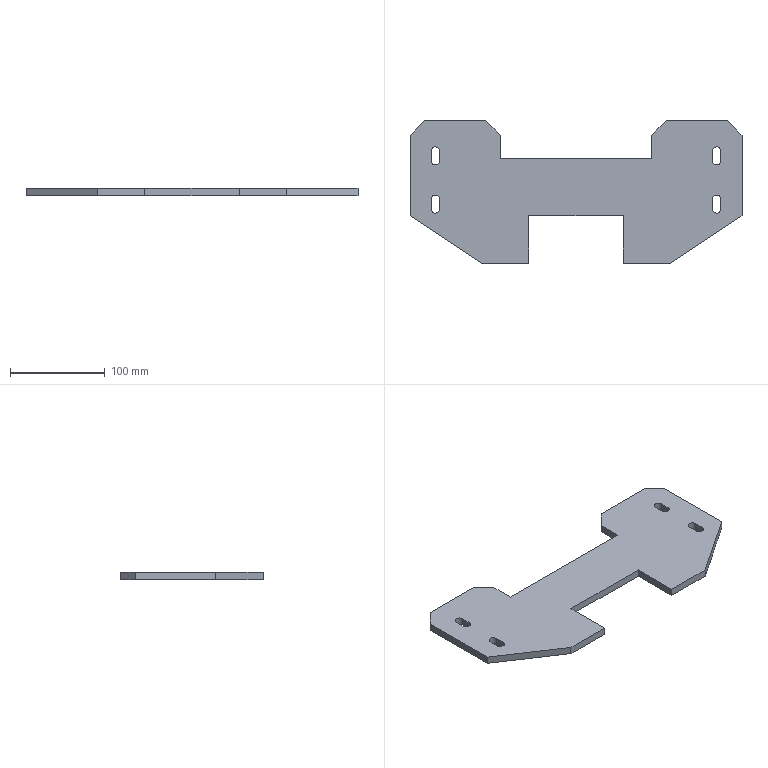Part | SolidWorks | features Extrusion 1 | 1 solid | 36 faces | box 350 x 150 x 8 mm | volume 290284 mm3 | plane 28 | cylinder 8 | commonest cylinder face diameters 9 x8
STEP:
#1=CARTESIAN_POINT('',(175.,-25.,8.));
#2=VERTEX_POINT('',#1);
#3=CARTESIAN_POINT('',(175.,60.,8.));
#4=VERTEX_POINT('',#3);
#5=CARTESIAN_POINT('',(175.,60.,8.));
#6=DIRECTION('',(0.,1.,0.));
#7=VECTOR('',#6,1000.);
#8=LINE('',#5,#7);
#9=EDGE_CURVE('',#2,#4,#8,.T.);
#10=ORIENTED_EDGE('',*,*,#9,.T.);
#11=CARTESIAN_POINT('',(160.,75.,8.));
#12=VERTEX_POINT('',#11);
#13=CARTESIAN_POINT('',(160.,75.,8.));
#14=DIRECTION('',(-0.7071,0.7071,0.));
#15=VECTOR('',#14,1000.);
#16=LINE('',#13,#15);
#17=EDGE_CURVE('',#4,#12,#16,.T.);
#18=ORIENTED_EDGE('',*,*,#17,.T.);
#19=CARTESIAN_POINT('',(95.,75.,8.));
#20=VERTEX_POINT('',#19);
#21=CARTESIAN_POINT('',(95.,75.,8.));
#22=DIRECTION('',(-1.,0.,0.));
#23=VECTOR('',#22,1000.);
#24=LINE('',#21,#23);
#25=EDGE_CURVE('',#12,#20,#24,.T.);
#26=ORIENTED_EDGE('',*,*,#25,.T.);
#27=CARTESIAN_POINT('',(80.,60.,8.));
#28=VERTEX_POINT('',#27);
#29=CARTESIAN_POINT('',(95.,75.,8.));
#30=DIRECTION('',(-0.7071,-0.7071,0.));
#31=VECTOR('',#30,1000.);
#32=LINE('',#29,#31);
#33=EDGE_CURVE('',#20,#28,#32,.T.);
#34=ORIENTED_EDGE('',*,*,#33,.T.);
#35=CARTESIAN_POINT('',(80.,35.,8.));
#36=VERTEX_POINT('',#35);
#37=CARTESIAN_POINT('',(80.,60.,8.));
#38=DIRECTION('',(0.,-1.,0.));
#39=VECTOR('',#38,1000.);
#40=LINE('',#37,#39);
#41=EDGE_CURVE('',#28,#36,#40,.T.);
#42=ORIENTED_EDGE('',*,*,#41,.T.);
#43=CARTESIAN_POINT('',(-80.,35.,8.));
#44=VERTEX_POINT('',#43);
#45=CARTESIAN_POINT('',(-80.,35.,8.));
#46=DIRECTION('',(-1.,0.,0.));
#47=VECTOR('',#46,1000.);
#48=LINE('',#45,#47);
#49=EDGE_CURVE('',#36,#44,#48,.T.);
#50=ORIENTED_EDGE('',*,*,#49,.T.);
#51=CARTESIAN_POINT('',(-80.,60.,8.));
#52=VERTEX_POINT('',#51);
#53=CARTESIAN_POINT('',(-80.,60.,8.));
#54=DIRECTION('',(0.,1.,0.));
#55=VECTOR('',#54,1000.);
#56=LINE('',#53,#55);
#57=EDGE_CURVE('',#44,#52,#56,.T.);
#58=ORIENTED_EDGE('',*,*,#57,.T.);
#59=CARTESIAN_POINT('',(-95.,75.,8.));
#60=VERTEX_POINT('',#59);
#61=CARTESIAN_POINT('',(-95.,75.,8.));
#62=DIRECTION('',(-0.7071,0.7071,0.));
#63=VECTOR('',#62,1000.);
#64=LINE('',#61,#63);
#65=EDGE_CURVE('',#52,#60,#64,.T.);
#66=ORIENTED_EDGE('',*,*,#65,.T.);
#67=CARTESIAN_POINT('',(-160.,75.,8.));
#68=VERTEX_POINT('',#67);
#69=CARTESIAN_POINT('',(-160.,75.,8.));
#70=DIRECTION('',(-1.,0.,0.));
#71=VECTOR('',#70,1000.);
#72=LINE('',#69,#71);
#73=EDGE_CURVE('',#60,#68,#72,.T.);
#74=ORIENTED_EDGE('',*,*,#73,.T.);
#75=CARTESIAN_POINT('',(-175.,60.,8.));
#76=VERTEX_POINT('',#75);
#77=CARTESIAN_POINT('',(-175.,60.,8.));
#78=DIRECTION('',(-0.7071,-0.7071,0.));
#79=VECTOR('',#78,1000.);
#80=LINE('',#77,#79);
#81=EDGE_CURVE('',#68,#76,#80,.T.);
#82=ORIENTED_EDGE('',*,*,#81,.T.);
#83=CARTESIAN_POINT('',(-175.,-25.,8.));
#84=VERTEX_POINT('',#83);
#85=CARTESIAN_POINT('',(-175.,60.,8.));
#86=DIRECTION('',(0.,-1.,0.));
#87=VECTOR('',#86,1000.);
#88=LINE('',#85,#87);
#89=EDGE_CURVE('',#76,#84,#88,.T.);
#90=ORIENTED_EDGE('',*,*,#89,.T.);
#91=CARTESIAN_POINT('',(-100.,-75.,8.));
#92=VERTEX_POINT('',#91);
#93=CARTESIAN_POINT('',(-175.,-25.,8.));
#94=DIRECTION('',(0.8321,-0.5547,0.));
#95=VECTOR('',#94,1000.);
#96=LINE('',#93,#95);
#97=EDGE_CURVE('',#84,#92,#96,.T.);
#98=ORIENTED_EDGE('',*,*,#97,.T.);
#99=CARTESIAN_POINT('',(-50.,-75.,8.));
#100=VERTEX_POINT('',#99);
#101=CARTESIAN_POINT('',(-100.,-75.,8.));
#102=DIRECTION('',(1.,0.,0.));
#103=VECTOR('',#102,1000.);
#104=LINE('',#101,#103);
#105=EDGE_CURVE('',#92,#100,#104,.T.);
#106=ORIENTED_EDGE('',*,*,#105,.T.);
#107=CARTESIAN_POINT('',(-50.,-25.,8.));
#108=VERTEX_POINT('',#107);
#109=CARTESIAN_POINT('',(-50.,-75.,8.));
#110=DIRECTION('',(0.,1.,0.));
#111=VECTOR('',#110,1000.);
#112=LINE('',#109,#111);
#113=EDGE_CURVE('',#100,#108,#112,.T.);
#114=ORIENTED_EDGE('',*,*,#113,.T.);
#115=CARTESIAN_POINT('',(50.,-25.,8.));
#116=VERTEX_POINT('',#115);
#117=CARTESIAN_POINT('',(-50.,-25.,8.));
#118=DIRECTION('',(1.,0.,0.));
#119=VECTOR('',#118,1000.);
#120=LINE('',#117,#119);
#121=EDGE_CURVE('',#108,#116,#120,.T.);
#122=ORIENTED_EDGE('',*,*,#121,.T.);
#123=CARTESIAN_POINT('',(50.,-75.,8.));
#124=VERTEX_POINT('',#123);
#125=CARTESIAN_POINT('',(50.,-25.,8.));
#126=DIRECTION('',(0.,-1.,0.));
#127=VECTOR('',#126,1000.);
#128=LINE('',#125,#127);
#129=EDGE_CURVE('',#116,#124,#128,.T.);
#130=ORIENTED_EDGE('',*,*,#129,.T.);
#131=CARTESIAN_POINT('',(100.,-75.,8.));
#132=VERTEX_POINT('',#131);
#133=CARTESIAN_POINT('',(50.,-75.,8.));
#134=DIRECTION('',(1.,0.,0.));
#135=VECTOR('',#134,1000.);
#136=LINE('',#133,#135);
#137=EDGE_CURVE('',#124,#132,#136,.T.);
#138=ORIENTED_EDGE('',*,*,#137,.T.);
#139=CARTESIAN_POINT('',(175.,-25.,8.));
#140=DIRECTION('',(0.8321,0.5547,0.));
#141=VECTOR('',#140,1000.);
#142=LINE('',#139,#141);
#143=EDGE_CURVE('',#132,#2,#142,.T.);
#144=ORIENTED_EDGE('',*,*,#143,.T.);
#145=EDGE_LOOP('',(#10,#18,#26,#34,#42,#50,#58,#66,#74,#82,#90,#98,#106,#114,#122,#130,#138,#144));
#146=FACE_OUTER_BOUND('',#145,.T.);
#147=CARTESIAN_POINT('',(-152.8,43.,8.));
#148=VERTEX_POINT('',#147);
#149=CARTESIAN_POINT('',(-152.8,33.,8.));
#150=VERTEX_POINT('',#149);
#151=CARTESIAN_POINT('',(-152.8,43.,8.));
#152=DIRECTION('',(0.,-1.,0.));
#153=VECTOR('',#152,1000.);
#154=LINE('',#151,#153);
#155=EDGE_CURVE('',#148,#150,#154,.T.);
#156=ORIENTED_EDGE('',*,*,#155,.F.);
#157=CARTESIAN_POINT('',(-143.8,43.,8.));
#158=VERTEX_POINT('',#157);
#159=CARTESIAN_POINT('',(-148.3,43.,8.));
#160=DIRECTION('',(0.,0.,1.));
#161=DIRECTION('',(1.,0.,0.));
#162=AXIS2_PLACEMENT_3D('',#159,#160,#161);
#163=CIRCLE('',#162,4.5);
#164=EDGE_CURVE('',#158,#148,#163,.T.);
#165=ORIENTED_EDGE('',*,*,#164,.F.);
#166=CARTESIAN_POINT('',(-143.8,33.,8.));
#167=VERTEX_POINT('',#166);
#168=CARTESIAN_POINT('',(-143.8,43.,8.));
#169=DIRECTION('',(0.,1.,0.));
#170=VECTOR('',#169,1000.);
#171=LINE('',#168,#170);
#172=EDGE_CURVE('',#167,#158,#171,.T.);
#173=ORIENTED_EDGE('',*,*,#172,.F.);
#174=CARTESIAN_POINT('',(-148.3,33.,8.));
#175=DIRECTION('',(0.,0.,1.));
#176=DIRECTION('',(1.,0.,0.));
#177=AXIS2_PLACEMENT_3D('',#174,#175,#176);
#178=CIRCLE('',#177,4.5);
#179=EDGE_CURVE('',#150,#167,#178,.T.);
#180=ORIENTED_EDGE('',*,*,#179,.F.);
#181=EDGE_LOOP('',(#156,#165,#173,#180));
#182=FACE_BOUND('',#181,.T.);
#183=CARTESIAN_POINT('',(-152.8,-7.8,8.));
#184=VERTEX_POINT('',#183);
#185=CARTESIAN_POINT('',(-152.8,-17.8,8.));
#186=VERTEX_POINT('',#185);
#187=CARTESIAN_POINT('',(-152.8,-7.8,8.));
#188=DIRECTION('',(0.,-1.,0.));
#189=VECTOR('',#188,1000.);
#190=LINE('',#187,#189);
#191=EDGE_CURVE('',#184,#186,#190,.T.);
#192=ORIENTED_EDGE('',*,*,#191,.F.);
#193=CARTESIAN_POINT('',(-143.8,-7.8,8.));
#194=VERTEX_POINT('',#193);
#195=CARTESIAN_POINT('',(-148.3,-7.8,8.));
#196=DIRECTION('',(0.,0.,1.));
#197=DIRECTION('',(1.,0.,0.));
#198=AXIS2_PLACEMENT_3D('',#195,#196,#197);
#199=CIRCLE('',#198,4.5);
#200=EDGE_CURVE('',#194,#184,#199,.T.);
#201=ORIENTED_EDGE('',*,*,#200,.F.);
#202=CARTESIAN_POINT('',(-143.8,-17.8,8.));
#203=VERTEX_POINT('',#202);
#204=CARTESIAN_POINT('',(-143.8,-7.8,8.));
#205=DIRECTION('',(0.,1.,0.));
#206=VECTOR('',#205,1000.);
#207=LINE('',#204,#206);
#208=EDGE_CURVE('',#203,#194,#207,.T.);
#209=ORIENTED_EDGE('',*,*,#208,.F.);
#210=CARTESIAN_POINT('',(-148.3,-17.8,8.));
#211=DIRECTION('',(0.,0.,1.));
#212=DIRECTION('',(1.,0.,0.));
#213=AXIS2_PLACEMENT_3D('',#210,#211,#212);
#214=CIRCLE('',#213,4.5);
#215=EDGE_CURVE('',#186,#203,#214,.T.);
#216=ORIENTED_EDGE('',*,*,#215,.F.);
#217=EDGE_LOOP('',(#192,#201,#209,#216));
#218=FACE_BOUND('',#217,.T.);
#219=CARTESIAN_POINT('',(143.8,-7.8,8.));
#220=VERTEX_POINT('',#219);
#221=CARTESIAN_POINT('',(143.8,-17.8,8.));
#222=VERTEX_POINT('',#221);
#223=CARTESIAN_POINT('',(143.8,-7.8,8.));
#224=DIRECTION('',(0.,-1.,0.));
#225=VECTOR('',#224,1000.);
#226=LINE('',#223,#225);
#227=EDGE_CURVE('',#220,#222,#226,.T.);
#228=ORIENTED_EDGE('',*,*,#227,.F.);
#229=CARTESIAN_POINT('',(152.8,-7.8,8.));
#230=VERTEX_POINT('',#229);
#231=CARTESIAN_POINT('',(148.3,-7.8,8.));
#232=DIRECTION('',(0.,0.,1.));
#233=DIRECTION('',(-1.,0.,0.));
#234=AXIS2_PLACEMENT_3D('',#231,#232,#233);
#235=CIRCLE('',#234,4.5);
#236=EDGE_CURVE('',#230,#220,#235,.T.);
#237=ORIENTED_EDGE('',*,*,#236,.F.);
#238=CARTESIAN_POINT('',(152.8,-17.8,8.));
#239=VERTEX_POINT('',#238);
#240=CARTESIAN_POINT('',(152.8,-7.8,8.));
#241=DIRECTION('',(0.,1.,0.));
#242=VECTOR('',#241,1000.);
#243=LINE('',#240,#242);
#244=EDGE_CURVE('',#239,#230,#243,.T.);
#245=ORIENTED_EDGE('',*,*,#244,.F.);
#246=CARTESIAN_POINT('',(148.3,-17.8,8.));
#247=DIRECTION('',(0.,0.,1.));
#248=DIRECTION('',(-1.,0.,0.));
#249=AXIS2_PLACEMENT_3D('',#246,#247,#248);
#250=CIRCLE('',#249,4.5);
#251=EDGE_CURVE('',#222,#239,#250,.T.);
#252=ORIENTED_EDGE('',*,*,#251,.F.);
#253=EDGE_LOOP('',(#228,#237,#245,#252));
#254=FACE_BOUND('',#253,.T.);
#255=CARTESIAN_POINT('',(143.8,43.,8.));
#256=VERTEX_POINT('',#255);
#257=CARTESIAN_POINT('',(143.8,33.,8.));
#258=VERTEX_POINT('',#257);
#259=CARTESIAN_POINT('',(143.8,43.,8.));
#260=DIRECTION('',(0.,-1.,0.));
#261=VECTOR('',#260,1000.);
#262=LINE('',#259,#261);
#263=EDGE_CURVE('',#256,#258,#262,.T.);
#264=ORIENTED_EDGE('',*,*,#263,.F.);
#265=CARTESIAN_POINT('',(152.8,43.,8.));
#266=VERTEX_POINT('',#265);
#267=CARTESIAN_POINT('',(148.3,43.,8.));
#268=DIRECTION('',(0.,0.,1.));
#269=DIRECTION('',(-1.,0.,0.));
#270=AXIS2_PLACEMENT_3D('',#267,#268,#269);
#271=CIRCLE('',#270,4.5);
#272=EDGE_CURVE('',#266,#256,#271,.T.);
#273=ORIENTED_EDGE('',*,*,#272,.F.);
#274=CARTESIAN_POINT('',(152.8,33.,8.));
#275=VERTEX_POINT('',#274);
#276=CARTESIAN_POINT('',(152.8,43.,8.));
#277=DIRECTION('',(0.,1.,0.));
#278=VECTOR('',#277,1000.);
#279=LINE('',#276,#278);
#280=EDGE_CURVE('',#275,#266,#279,.T.);
#281=ORIENTED_EDGE('',*,*,#280,.F.);
#282=CARTESIAN_POINT('',(148.3,33.,8.));
#283=DIRECTION('',(0.,0.,1.));
#284=DIRECTION('',(-1.,0.,0.));
#285=AXIS2_PLACEMENT_3D('',#282,#283,#284);
#286=CIRCLE('',#285,4.5);
#287=EDGE_CURVE('',#258,#275,#286,.T.);
#288=ORIENTED_EDGE('',*,*,#287,.F.);
#289=EDGE_LOOP('',(#264,#273,#281,#288));
#290=FACE_BOUND('',#289,.T.);
#291=CARTESIAN_POINT('',(0.,0.,8.));
#292=DIRECTION('',(0.,0.,1.));
#293=DIRECTION('',(1.,0.,0.));
#294=AXIS2_PLACEMENT_3D('',#291,#292,#293);
#295=PLANE('',#294);
#296=ADVANCED_FACE('',(#146,#182,#218,#254,#290),#295,.T.);
#297=CARTESIAN_POINT('',(152.8,-7.8,0.));
#298=VERTEX_POINT('',#297);
#299=CARTESIAN_POINT('',(143.8,-7.8,0.));
#300=VERTEX_POINT('',#299);
#301=CARTESIAN_POINT('',(148.3,-7.8,0.));
#302=DIRECTION('',(0.,0.,1.));
#303=DIRECTION('',(-1.,0.,0.));
#304=AXIS2_PLACEMENT_3D('',#301,#302,#303);
#305=CIRCLE('',#304,4.5);
#306=EDGE_CURVE('',#298,#300,#305,.T.);
#307=ORIENTED_EDGE('',*,*,#306,.T.);
#308=CARTESIAN_POINT('',(143.8,-17.8,0.));
#309=VERTEX_POINT('',#308);
#310=CARTESIAN_POINT('',(143.8,-7.8,0.));
#311=DIRECTION('',(0.,-1.,0.));
#312=VECTOR('',#311,1000.);
#313=LINE('',#310,#312);
#314=EDGE_CURVE('',#300,#309,#313,.T.);
#315=ORIENTED_EDGE('',*,*,#314,.T.);
#316=CARTESIAN_POINT('',(152.8,-17.8,0.));
#317=VERTEX_POINT('',#316);
#318=CARTESIAN_POINT('',(148.3,-17.8,0.));
#319=DIRECTION('',(0.,0.,1.));
#320=DIRECTION('',(-1.,0.,0.));
#321=AXIS2_PLACEMENT_3D('',#318,#319,#320);
#322=CIRCLE('',#321,4.5);
#323=EDGE_CURVE('',#309,#317,#322,.T.);
#324=ORIENTED_EDGE('',*,*,#323,.T.);
#325=CARTESIAN_POINT('',(152.8,-7.8,0.));
#326=DIRECTION('',(0.,1.,0.));
#327=VECTOR('',#326,1000.);
#328=LINE('',#325,#327);
#329=EDGE_CURVE('',#317,#298,#328,.T.);
#330=ORIENTED_EDGE('',*,*,#329,.T.);
#331=EDGE_LOOP('',(#307,#315,#324,#330));
#332=FACE_BOUND('',#331,.T.);
#333=CARTESIAN_POINT('',(-143.8,43.,0.));
#334=VERTEX_POINT('',#333);
#335=CARTESIAN_POINT('',(-152.8,43.,0.));
#336=VERTEX_POINT('',#335);
#337=CARTESIAN_POINT('',(-148.3,43.,0.));
#338=DIRECTION('',(0.,0.,1.));
#339=DIRECTION('',(1.,0.,0.));
#340=AXIS2_PLACEMENT_3D('',#337,#338,#339);
#341=CIRCLE('',#340,4.5);
#342=EDGE_CURVE('',#334,#336,#341,.T.);
#343=ORIENTED_EDGE('',*,*,#342,.T.);
#344=CARTESIAN_POINT('',(-152.8,33.,0.));
#345=VERTEX_POINT('',#344);
#346=CARTESIAN_POINT('',(-152.8,43.,0.));
#347=DIRECTION('',(0.,-1.,0.));
#348=VECTOR('',#347,1000.);
#349=LINE('',#346,#348);
#350=EDGE_CURVE('',#336,#345,#349,.T.);
#351=ORIENTED_EDGE('',*,*,#350,.T.);
#352=CARTESIAN_POINT('',(-143.8,33.,0.));
#353=VERTEX_POINT('',#352);
#354=CARTESIAN_POINT('',(-148.3,33.,0.));
#355=DIRECTION('',(0.,0.,1.));
#356=DIRECTION('',(1.,0.,0.));
#357=AXIS2_PLACEMENT_3D('',#354,#355,#356);
#358=CIRCLE('',#357,4.5);
#359=EDGE_CURVE('',#345,#353,#358,.T.);
#360=ORIENTED_EDGE('',*,*,#359,.T.);
#361=CARTESIAN_POINT('',(-143.8,43.,0.));
#362=DIRECTION('',(0.,1.,0.));
#363=VECTOR('',#362,1000.);
#364=LINE('',#361,#363);
#365=EDGE_CURVE('',#353,#334,#364,.T.);
#366=ORIENTED_EDGE('',*,*,#365,.T.);
#367=EDGE_LOOP('',(#343,#351,#360,#366));
#368=FACE_BOUND('',#367,.T.);
#369=CARTESIAN_POINT('',(175.,-25.,0.));
#370=VERTEX_POINT('',#369);
#371=CARTESIAN_POINT('',(175.,60.,0.));
#372=VERTEX_POINT('',#371);
#373=CARTESIAN_POINT('',(175.,60.,0.));
#374=DIRECTION('',(0.,1.,0.));
#375=VECTOR('',#374,1000.);
#376=LINE('',#373,#375);
#377=EDGE_CURVE('',#370,#372,#376,.T.);
#378=ORIENTED_EDGE('',*,*,#377,.F.);
#379=CARTESIAN_POINT('',(100.,-75.,0.));
#380=VERTEX_POINT('',#379);
#381=CARTESIAN_POINT('',(175.,-25.,0.));
#382=DIRECTION('',(0.8321,0.5547,0.));
#383=VECTOR('',#382,1000.);
#384=LINE('',#381,#383);
#385=EDGE_CURVE('',#380,#370,#384,.T.);
#386=ORIENTED_EDGE('',*,*,#385,.F.);
#387=CARTESIAN_POINT('',(50.,-75.,0.));
#388=VERTEX_POINT('',#387);
#389=CARTESIAN_POINT('',(50.,-75.,0.));
#390=DIRECTION('',(1.,0.,0.));
#391=VECTOR('',#390,1000.);
#392=LINE('',#389,#391);
#393=EDGE_CURVE('',#388,#380,#392,.T.);
#394=ORIENTED_EDGE('',*,*,#393,.F.);
#395=CARTESIAN_POINT('',(50.,-25.,0.));
#396=VERTEX_POINT('',#395);
#397=CARTESIAN_POINT('',(50.,-25.,0.));
#398=DIRECTION('',(0.,-1.,0.));
#399=VECTOR('',#398,1000.);
#400=LINE('',#397,#399);
#401=EDGE_CURVE('',#396,#388,#400,.T.);
#402=ORIENTED_EDGE('',*,*,#401,.F.);
#403=CARTESIAN_POINT('',(-50.,-25.,0.));
#404=VERTEX_POINT('',#403);
#405=CARTESIAN_POINT('',(-50.,-25.,0.));
#406=DIRECTION('',(1.,0.,0.));
#407=VECTOR('',#406,1000.);
#408=LINE('',#405,#407);
#409=EDGE_CURVE('',#404,#396,#408,.T.);
#410=ORIENTED_EDGE('',*,*,#409,.F.);
#411=CARTESIAN_POINT('',(-50.,-75.,0.));
#412=VERTEX_POINT('',#411);
#413=CARTESIAN_POINT('',(-50.,-75.,0.));
#414=DIRECTION('',(0.,1.,0.));
#415=VECTOR('',#414,1000.);
#416=LINE('',#413,#415);
#417=EDGE_CURVE('',#412,#404,#416,.T.);
#418=ORIENTED_EDGE('',*,*,#417,.F.);
#419=CARTESIAN_POINT('',(-100.,-75.,0.));
#420=VERTEX_POINT('',#419);
#421=CARTESIAN_POINT('',(-100.,-75.,0.));
#422=DIRECTION('',(1.,0.,0.));
#423=VECTOR('',#422,1000.);
#424=LINE('',#421,#423);
#425=EDGE_CURVE('',#420,#412,#424,.T.);
#426=ORIENTED_EDGE('',*,*,#425,.F.);
#427=CARTESIAN_POINT('',(-175.,-25.,0.));
#428=VERTEX_POINT('',#427);
#429=CARTESIAN_POINT('',(-175.,-25.,0.));
#430=DIRECTION('',(0.8321,-0.5547,0.));
#431=VECTOR('',#430,1000.);
#432=LINE('',#429,#431);
#433=EDGE_CURVE('',#428,#420,#432,.T.);
#434=ORIENTED_EDGE('',*,*,#433,.F.);
#435=CARTESIAN_POINT('',(-175.,60.,0.));
#436=VERTEX_POINT('',#435);
#437=CARTESIAN_POINT('',(-175.,60.,0.));
#438=DIRECTION('',(0.,-1.,0.));
#439=VECTOR('',#438,1000.);
#440=LINE('',#437,#439);
#441=EDGE_CURVE('',#436,#428,#440,.T.);
#442=ORIENTED_EDGE('',*,*,#441,.F.);
#443=CARTESIAN_POINT('',(-160.,75.,0.));
#444=VERTEX_POINT('',#443);
#445=CARTESIAN_POINT('',(-175.,60.,0.));
#446=DIRECTION('',(-0.7071,-0.7071,0.));
#447=VECTOR('',#446,1000.);
#448=LINE('',#445,#447);
#449=EDGE_CURVE('',#444,#436,#448,.T.);
#450=ORIENTED_EDGE('',*,*,#449,.F.);
#451=CARTESIAN_POINT('',(-95.,75.,0.));
#452=VERTEX_POINT('',#451);
#453=CARTESIAN_POINT('',(-160.,75.,0.));
#454=DIRECTION('',(-1.,0.,0.));
#455=VECTOR('',#454,1000.);
#456=LINE('',#453,#455);
#457=EDGE_CURVE('',#452,#444,#456,.T.);
#458=ORIENTED_EDGE('',*,*,#457,.F.);
#459=CARTESIAN_POINT('',(-80.,60.,0.));
#460=VERTEX_POINT('',#459);
#461=CARTESIAN_POINT('',(-95.,75.,0.));
#462=DIRECTION('',(-0.7071,0.7071,0.));
#463=VECTOR('',#462,1000.);
#464=LINE('',#461,#463);
#465=EDGE_CURVE('',#460,#452,#464,.T.);
#466=ORIENTED_EDGE('',*,*,#465,.F.);
#467=CARTESIAN_POINT('',(-80.,35.,0.));
#468=VERTEX_POINT('',#467);
#469=CARTESIAN_POINT('',(-80.,60.,0.));
#470=DIRECTION('',(0.,1.,0.));
#471=VECTOR('',#470,1000.);
#472=LINE('',#469,#471);
#473=EDGE_CURVE('',#468,#460,#472,.T.);
#474=ORIENTED_EDGE('',*,*,#473,.F.);
#475=CARTESIAN_POINT('',(80.,35.,0.));
#476=VERTEX_POINT('',#475);
#477=CARTESIAN_POINT('',(-80.,35.,0.));
#478=DIRECTION('',(-1.,0.,0.));
#479=VECTOR('',#478,1000.);
#480=LINE('',#477,#479);
#481=EDGE_CURVE('',#476,#468,#480,.T.);
#482=ORIENTED_EDGE('',*,*,#481,.F.);
#483=CARTESIAN_POINT('',(80.,60.,0.));
#484=VERTEX_POINT('',#483);
#485=CARTESIAN_POINT('',(80.,60.,0.));
#486=DIRECTION('',(0.,-1.,0.));
#487=VECTOR('',#486,1000.);
#488=LINE('',#485,#487);
#489=EDGE_CURVE('',#484,#476,#488,.T.);
#490=ORIENTED_EDGE('',*,*,#489,.F.);
#491=CARTESIAN_POINT('',(95.,75.,0.));
#492=VERTEX_POINT('',#491);
#493=CARTESIAN_POINT('',(95.,75.,0.));
#494=DIRECTION('',(-0.7071,-0.7071,0.));
#495=VECTOR('',#494,1000.);
#496=LINE('',#493,#495);
#497=EDGE_CURVE('',#492,#484,#496,.T.);
#498=ORIENTED_EDGE('',*,*,#497,.F.);
#499=CARTESIAN_POINT('',(160.,75.,0.));
#500=VERTEX_POINT('',#499);
#501=CARTESIAN_POINT('',(95.,75.,0.));
#502=DIRECTION('',(-1.,0.,0.));
#503=VECTOR('',#502,1000.);
#504=LINE('',#501,#503);
#505=EDGE_CURVE('',#500,#492,#504,.T.);
#506=ORIENTED_EDGE('',*,*,#505,.F.);
#507=CARTESIAN_POINT('',(160.,75.,0.));
#508=DIRECTION('',(-0.7071,0.7071,0.));
#509=VECTOR('',#508,1000.);
#510=LINE('',#507,#509);
#511=EDGE_CURVE('',#372,#500,#510,.T.);
#512=ORIENTED_EDGE('',*,*,#511,.F.);
#513=EDGE_LOOP('',(#378,#386,#394,#402,#410,#418,#426,#434,#442,#450,#458,#466,#474,#482,#490,#498,#506,#512));
#514=FACE_OUTER_BOUND('',#513,.T.);
#515=CARTESIAN_POINT('',(-143.8,-7.8,0.));
#516=VERTEX_POINT('',#515);
#517=CARTESIAN_POINT('',(-152.8,-7.8,0.));
#518=VERTEX_POINT('',#517);
#519=CARTESIAN_POINT('',(-148.3,-7.8,0.));
#520=DIRECTION('',(0.,0.,1.));
#521=DIRECTION('',(1.,0.,0.));
#522=AXIS2_PLACEMENT_3D('',#519,#520,#521);
#523=CIRCLE('',#522,4.5);
#524=EDGE_CURVE('',#516,#518,#523,.T.);
#525=ORIENTED_EDGE('',*,*,#524,.T.);
#526=CARTESIAN_POINT('',(-152.8,-17.8,0.));
#527=VERTEX_POINT('',#526);
#528=CARTESIAN_POINT('',(-152.8,-7.8,0.));
#529=DIRECTION('',(0.,-1.,0.));
#530=VECTOR('',#529,1000.);
#531=LINE('',#528,#530);
#532=EDGE_CURVE('',#518,#527,#531,.T.);
#533=ORIENTED_EDGE('',*,*,#532,.T.);
#534=CARTESIAN_POINT('',(-143.8,-17.8,0.));
#535=VERTEX_POINT('',#534);
#536=CARTESIAN_POINT('',(-148.3,-17.8,0.));
#537=DIRECTION('',(0.,0.,1.));
#538=DIRECTION('',(1.,0.,0.));
#539=AXIS2_PLACEMENT_3D('',#536,#537,#538);
#540=CIRCLE('',#539,4.5);
#541=EDGE_CURVE('',#527,#535,#540,.T.);
#542=ORIENTED_EDGE('',*,*,#541,.T.);
#543=CARTESIAN_POINT('',(-143.8,-7.8,0.));
#544=DIRECTION('',(0.,1.,0.));
#545=VECTOR('',#544,1000.);
#546=LINE('',#543,#545);
#547=EDGE_CURVE('',#535,#516,#546,.T.);
#548=ORIENTED_EDGE('',*,*,#547,.T.);
#549=EDGE_LOOP('',(#525,#533,#542,#548));
#550=FACE_BOUND('',#549,.T.);
#551=CARTESIAN_POINT('',(152.8,43.,0.));
#552=VERTEX_POINT('',#551);
#553=CARTESIAN_POINT('',(143.8,43.,0.));
#554=VERTEX_POINT('',#553);
#555=CARTESIAN_POINT('',(148.3,43.,0.));
#556=DIRECTION('',(0.,0.,1.));
#557=DIRECTION('',(-1.,0.,0.));
#558=AXIS2_PLACEMENT_3D('',#555,#556,#557);
#559=CIRCLE('',#558,4.5);
#560=EDGE_CURVE('',#552,#554,#559,.T.);
#561=ORIENTED_EDGE('',*,*,#560,.T.);
#562=CARTESIAN_POINT('',(143.8,33.,0.));
#563=VERTEX_POINT('',#562);
#564=CARTESIAN_POINT('',(143.8,43.,0.));
#565=DIRECTION('',(0.,-1.,0.));
#566=VECTOR('',#565,1000.);
#567=LINE('',#564,#566);
#568=EDGE_CURVE('',#554,#563,#567,.T.);
#569=ORIENTED_EDGE('',*,*,#568,.T.);
#570=CARTESIAN_POINT('',(152.8,33.,0.));
#571=VERTEX_POINT('',#570);
#572=CARTESIAN_POINT('',(148.3,33.,0.));
#573=DIRECTION('',(0.,0.,1.));
#574=DIRECTION('',(-1.,0.,0.));
#575=AXIS2_PLACEMENT_3D('',#572,#573,#574);
#576=CIRCLE('',#575,4.5);
#577=EDGE_CURVE('',#563,#571,#576,.T.);
#578=ORIENTED_EDGE('',*,*,#577,.T.);
#579=CARTESIAN_POINT('',(152.8,43.,0.));
#580=DIRECTION('',(0.,1.,0.));
#581=VECTOR('',#580,1000.);
#582=LINE('',#579,#581);
#583=EDGE_CURVE('',#571,#552,#582,.T.);
#584=ORIENTED_EDGE('',*,*,#583,.T.);
#585=EDGE_LOOP('',(#561,#569,#578,#584));
#586=FACE_BOUND('',#585,.T.);
#587=CARTESIAN_POINT('',(0.,0.,0.));
#588=DIRECTION('',(0.,0.,1.));
#589=DIRECTION('',(1.,0.,0.));
#590=AXIS2_PLACEMENT_3D('',#587,#588,#589);
#591=PLANE('',#590);
#592=ADVANCED_FACE('',(#332,#368,#514,#550,#586),#591,.F.);
#593=ORIENTED_EDGE('',*,*,#377,.T.);
#594=CARTESIAN_POINT('',(175.,60.,8.));
#595=DIRECTION('',(0.,0.,-1.));
#596=VECTOR('',#595,1000.);
#597=LINE('',#594,#596);
#598=EDGE_CURVE('',#4,#372,#597,.T.);
#599=ORIENTED_EDGE('',*,*,#598,.F.);
#600=ORIENTED_EDGE('',*,*,#9,.F.);
#601=CARTESIAN_POINT('',(175.,-25.,8.));
#602=DIRECTION('',(0.,0.,-1.));
#603=VECTOR('',#602,1000.);
#604=LINE('',#601,#603);
#605=EDGE_CURVE('',#2,#370,#604,.T.);
#606=ORIENTED_EDGE('',*,*,#605,.T.);
#607=EDGE_LOOP('',(#593,#599,#600,#606));
#608=FACE_OUTER_BOUND('',#607,.T.);
#609=CARTESIAN_POINT('',(175.,60.,8.));
#610=DIRECTION('',(-1.,0.,0.));
#611=DIRECTION('',(0.,0.,1.));
#612=AXIS2_PLACEMENT_3D('',#609,#610,#611);
#613=PLANE('',#612);
#614=ADVANCED_FACE('',(#608),#613,.F.);
#615=ORIENTED_EDGE('',*,*,#511,.T.);
#616=CARTESIAN_POINT('',(160.,75.,8.));
#617=DIRECTION('',(0.,0.,-1.));
#618=VECTOR('',#617,1000.);
#619=LINE('',#616,#618);
#620=EDGE_CURVE('',#12,#500,#619,.T.);
#621=ORIENTED_EDGE('',*,*,#620,.F.);
#622=ORIENTED_EDGE('',*,*,#17,.F.);
#623=ORIENTED_EDGE('',*,*,#598,.T.);
#624=EDGE_LOOP('',(#615,#621,#622,#623));
#625=FACE_OUTER_BOUND('',#624,.T.);
#626=CARTESIAN_POINT('',(160.,75.,8.));
#627=DIRECTION('',(-0.7071,-0.7071,0.));
#628=DIRECTION('',(0.7071,-0.7071,0.));
#629=AXIS2_PLACEMENT_3D('',#626,#627,#628);
#630=PLANE('',#629);
#631=ADVANCED_FACE('',(#625),#630,.F.);
#632=ORIENTED_EDGE('',*,*,#505,.T.);
#633=CARTESIAN_POINT('',(95.,75.,8.));
#634=DIRECTION('',(0.,0.,-1.));
#635=VECTOR('',#634,1000.);
#636=LINE('',#633,#635);
#637=EDGE_CURVE('',#20,#492,#636,.T.);
#638=ORIENTED_EDGE('',*,*,#637,.F.);
#639=ORIENTED_EDGE('',*,*,#25,.F.);
#640=ORIENTED_EDGE('',*,*,#620,.T.);
#641=EDGE_LOOP('',(#632,#638,#639,#640));
#642=FACE_OUTER_BOUND('',#641,.T.);
#643=CARTESIAN_POINT('',(95.,75.,8.));
#644=DIRECTION('',(0.,-1.,0.));
#645=DIRECTION('',(0.,0.,-1.));
#646=AXIS2_PLACEMENT_3D('',#643,#644,#645);
#647=PLANE('',#646);
#648=ADVANCED_FACE('',(#642),#647,.F.);
#649=ORIENTED_EDGE('',*,*,#497,.T.);
#650=CARTESIAN_POINT('',(80.,60.,8.));
#651=DIRECTION('',(0.,0.,-1.));
#652=VECTOR('',#651,1000.);
#653=LINE('',#650,#652);
#654=EDGE_CURVE('',#28,#484,#653,.T.);
#655=ORIENTED_EDGE('',*,*,#654,.F.);
#656=ORIENTED_EDGE('',*,*,#33,.F.);
#657=ORIENTED_EDGE('',*,*,#637,.T.);
#658=EDGE_LOOP('',(#649,#655,#656,#657));
#659=FACE_OUTER_BOUND('',#658,.T.);
#660=CARTESIAN_POINT('',(95.,75.,8.));
#661=DIRECTION('',(0.7071,-0.7071,0.));
#662=DIRECTION('',(0.7071,0.7071,0.));
#663=AXIS2_PLACEMENT_3D('',#660,#661,#662);
#664=PLANE('',#663);
#665=ADVANCED_FACE('',(#659),#664,.F.);
#666=ORIENTED_EDGE('',*,*,#489,.T.);
#667=CARTESIAN_POINT('',(80.,35.,8.));
#668=DIRECTION('',(0.,0.,-1.));
#669=VECTOR('',#668,1000.);
#670=LINE('',#667,#669);
#671=EDGE_CURVE('',#36,#476,#670,.T.);
#672=ORIENTED_EDGE('',*,*,#671,.F.);
#673=ORIENTED_EDGE('',*,*,#41,.F.);
#674=ORIENTED_EDGE('',*,*,#654,.T.);
#675=EDGE_LOOP('',(#666,#672,#673,#674));
#676=FACE_OUTER_BOUND('',#675,.T.);
#677=CARTESIAN_POINT('',(80.,60.,8.));
#678=DIRECTION('',(1.,0.,0.));
#679=DIRECTION('',(0.,1.,0.));
#680=AXIS2_PLACEMENT_3D('',#677,#678,#679);
#681=PLANE('',#680);
#682=ADVANCED_FACE('',(#676),#681,.F.);
#683=ORIENTED_EDGE('',*,*,#481,.T.);
#684=CARTESIAN_POINT('',(-80.,35.,8.));
#685=DIRECTION('',(0.,0.,-1.));
#686=VECTOR('',#685,1000.);
#687=LINE('',#684,#686);
#688=EDGE_CURVE('',#44,#468,#687,.T.);
#689=ORIENTED_EDGE('',*,*,#688,.F.);
#690=ORIENTED_EDGE('',*,*,#49,.F.);
#691=ORIENTED_EDGE('',*,*,#671,.T.);
#692=EDGE_LOOP('',(#683,#689,#690,#691));
#693=FACE_OUTER_BOUND('',#692,.T.);
#694=CARTESIAN_POINT('',(-80.,35.,8.));
#695=DIRECTION('',(0.,-1.,0.));
#696=DIRECTION('',(0.,0.,-1.));
#697=AXIS2_PLACEMENT_3D('',#694,#695,#696);
#698=PLANE('',#697);
#699=ADVANCED_FACE('',(#693),#698,.F.);
#700=ORIENTED_EDGE('',*,*,#473,.T.);
#701=CARTESIAN_POINT('',(-80.,60.,8.));
#702=DIRECTION('',(0.,0.,-1.));
#703=VECTOR('',#702,1000.);
#704=LINE('',#701,#703);
#705=EDGE_CURVE('',#52,#460,#704,.T.);
#706=ORIENTED_EDGE('',*,*,#705,.F.);
#707=ORIENTED_EDGE('',*,*,#57,.F.);
#708=ORIENTED_EDGE('',*,*,#688,.T.);
#709=EDGE_LOOP('',(#700,#706,#707,#708));
#710=FACE_OUTER_BOUND('',#709,.T.);
#711=CARTESIAN_POINT('',(-80.,60.,8.));
#712=DIRECTION('',(-1.,0.,0.));
#713=DIRECTION('',(0.,0.,1.));
#714=AXIS2_PLACEMENT_3D('',#711,#712,#713);
#715=PLANE('',#714);
#716=ADVANCED_FACE('',(#710),#715,.F.);
#717=ORIENTED_EDGE('',*,*,#465,.T.);
#718=CARTESIAN_POINT('',(-95.,75.,8.));
#719=DIRECTION('',(0.,0.,-1.));
#720=VECTOR('',#719,1000.);
#721=LINE('',#718,#720);
#722=EDGE_CURVE('',#60,#452,#721,.T.);
#723=ORIENTED_EDGE('',*,*,#722,.F.);
#724=ORIENTED_EDGE('',*,*,#65,.F.);
#725=ORIENTED_EDGE('',*,*,#705,.T.);
#726=EDGE_LOOP('',(#717,#723,#724,#725));
#727=FACE_OUTER_BOUND('',#726,.T.);
#728=CARTESIAN_POINT('',(-95.,75.,8.));
#729=DIRECTION('',(-0.7071,-0.7071,0.));
#730=DIRECTION('',(0.7071,-0.7071,0.));
#731=AXIS2_PLACEMENT_3D('',#728,#729,#730);
#732=PLANE('',#731);
#733=ADVANCED_FACE('',(#727),#732,.F.);
#734=ORIENTED_EDGE('',*,*,#457,.T.);
#735=CARTESIAN_POINT('',(-160.,75.,8.));
#736=DIRECTION('',(0.,0.,-1.));
#737=VECTOR('',#736,1000.);
#738=LINE('',#735,#737);
#739=EDGE_CURVE('',#68,#444,#738,.T.);
#740=ORIENTED_EDGE('',*,*,#739,.F.);
#741=ORIENTED_EDGE('',*,*,#73,.F.);
#742=ORIENTED_EDGE('',*,*,#722,.T.);
#743=EDGE_LOOP('',(#734,#740,#741,#742));
#744=FACE_OUTER_BOUND('',#743,.T.);
#745=CARTESIAN_POINT('',(-160.,75.,8.));
#746=DIRECTION('',(0.,-1.,0.));
#747=DIRECTION('',(0.,0.,-1.));
#748=AXIS2_PLACEMENT_3D('',#745,#746,#747);
#749=PLANE('',#748);
#750=ADVANCED_FACE('',(#744),#749,.F.);
#751=ORIENTED_EDGE('',*,*,#449,.T.);
#752=CARTESIAN_POINT('',(-175.,60.,8.));
#753=DIRECTION('',(0.,0.,-1.));
#754=VECTOR('',#753,1000.);
#755=LINE('',#752,#754);
#756=EDGE_CURVE('',#76,#436,#755,.T.);
#757=ORIENTED_EDGE('',*,*,#756,.F.);
#758=ORIENTED_EDGE('',*,*,#81,.F.);
#759=ORIENTED_EDGE('',*,*,#739,.T.);
#760=EDGE_LOOP('',(#751,#757,#758,#759));
#761=FACE_OUTER_BOUND('',#760,.T.);
#762=CARTESIAN_POINT('',(-175.,60.,8.));
#763=DIRECTION('',(0.7071,-0.7071,0.));
#764=DIRECTION('',(0.7071,0.7071,0.));
#765=AXIS2_PLACEMENT_3D('',#762,#763,#764);
#766=PLANE('',#765);
#767=ADVANCED_FACE('',(#761),#766,.F.);
#768=ORIENTED_EDGE('',*,*,#441,.T.);
#769=CARTESIAN_POINT('',(-175.,-25.,8.));
#770=DIRECTION('',(0.,0.,-1.));
#771=VECTOR('',#770,1000.);
#772=LINE('',#769,#771);
#773=EDGE_CURVE('',#84,#428,#772,.T.);
#774=ORIENTED_EDGE('',*,*,#773,.F.);
#775=ORIENTED_EDGE('',*,*,#89,.F.);
#776=ORIENTED_EDGE('',*,*,#756,.T.);
#777=EDGE_LOOP('',(#768,#774,#775,#776));
#778=FACE_OUTER_BOUND('',#777,.T.);
#779=CARTESIAN_POINT('',(-175.,60.,8.));
#780=DIRECTION('',(1.,0.,0.));
#781=DIRECTION('',(0.,0.,-1.));
#782=AXIS2_PLACEMENT_3D('',#779,#780,#781);
#783=PLANE('',#782);
#784=ADVANCED_FACE('',(#778),#783,.F.);
#785=ORIENTED_EDGE('',*,*,#433,.T.);
#786=CARTESIAN_POINT('',(-100.,-75.,8.));
#787=DIRECTION('',(0.,0.,-1.));
#788=VECTOR('',#787,1000.);
#789=LINE('',#786,#788);
#790=EDGE_CURVE('',#92,#420,#789,.T.);
#791=ORIENTED_EDGE('',*,*,#790,.F.);
#792=ORIENTED_EDGE('',*,*,#97,.F.);
#793=ORIENTED_EDGE('',*,*,#773,.T.);
#794=EDGE_LOOP('',(#785,#791,#792,#793));
#795=FACE_OUTER_BOUND('',#794,.T.);
#796=CARTESIAN_POINT('',(-175.,-25.,8.));
#797=DIRECTION('',(0.5547,0.8321,0.));
#798=DIRECTION('',(-0.8321,0.5547,0.));
#799=AXIS2_PLACEMENT_3D('',#796,#797,#798);
#800=PLANE('',#799);
#801=ADVANCED_FACE('',(#795),#800,.F.);
#802=ORIENTED_EDGE('',*,*,#425,.T.);
#803=CARTESIAN_POINT('',(-50.,-75.,8.));
#804=DIRECTION('',(0.,0.,-1.));
#805=VECTOR('',#804,1000.);
#806=LINE('',#803,#805);
#807=EDGE_CURVE('',#100,#412,#806,.T.);
#808=ORIENTED_EDGE('',*,*,#807,.F.);
#809=ORIENTED_EDGE('',*,*,#105,.F.);
#810=ORIENTED_EDGE('',*,*,#790,.T.);
#811=EDGE_LOOP('',(#802,#808,#809,#810));
#812=FACE_OUTER_BOUND('',#811,.T.);
#813=CARTESIAN_POINT('',(-100.,-75.,8.));
#814=DIRECTION('',(0.,1.,0.));
#815=DIRECTION('',(0.,0.,1.));
#816=AXIS2_PLACEMENT_3D('',#813,#814,#815);
#817=PLANE('',#816);
#818=ADVANCED_FACE('',(#812),#817,.F.);
#819=ORIENTED_EDGE('',*,*,#417,.T.);
#820=CARTESIAN_POINT('',(-50.,-25.,8.));
#821=DIRECTION('',(0.,0.,-1.));
#822=VECTOR('',#821,1000.);
#823=LINE('',#820,#822);
#824=EDGE_CURVE('',#108,#404,#823,.T.);
#825=ORIENTED_EDGE('',*,*,#824,.F.);
#826=ORIENTED_EDGE('',*,*,#113,.F.);
#827=ORIENTED_EDGE('',*,*,#807,.T.);
#828=EDGE_LOOP('',(#819,#825,#826,#827));
#829=FACE_OUTER_BOUND('',#828,.T.);
#830=CARTESIAN_POINT('',(-50.,-75.,8.));
#831=DIRECTION('',(-1.,0.,0.));
#832=DIRECTION('',(0.,0.,1.));
#833=AXIS2_PLACEMENT_3D('',#830,#831,#832);
#834=PLANE('',#833);
#835=ADVANCED_FACE('',(#829),#834,.F.);
#836=ORIENTED_EDGE('',*,*,#409,.T.);
#837=CARTESIAN_POINT('',(50.,-25.,8.));
#838=DIRECTION('',(0.,0.,-1.));
#839=VECTOR('',#838,1000.);
#840=LINE('',#837,#839);
#841=EDGE_CURVE('',#116,#396,#840,.T.);
#842=ORIENTED_EDGE('',*,*,#841,.F.);
#843=ORIENTED_EDGE('',*,*,#121,.F.);
#844=ORIENTED_EDGE('',*,*,#824,.T.);
#845=EDGE_LOOP('',(#836,#842,#843,#844));
#846=FACE_OUTER_BOUND('',#845,.T.);
#847=CARTESIAN_POINT('',(-50.,-25.,8.));
#848=DIRECTION('',(0.,1.,0.));
#849=DIRECTION('',(0.,0.,1.));
#850=AXIS2_PLACEMENT_3D('',#847,#848,#849);
#851=PLANE('',#850);
#852=ADVANCED_FACE('',(#846),#851,.F.);
#853=ORIENTED_EDGE('',*,*,#401,.T.);
#854=CARTESIAN_POINT('',(50.,-75.,8.));
#855=DIRECTION('',(0.,0.,-1.));
#856=VECTOR('',#855,1000.);
#857=LINE('',#854,#856);
#858=EDGE_CURVE('',#124,#388,#857,.T.);
#859=ORIENTED_EDGE('',*,*,#858,.F.);
#860=ORIENTED_EDGE('',*,*,#129,.F.);
#861=ORIENTED_EDGE('',*,*,#841,.T.);
#862=EDGE_LOOP('',(#853,#859,#860,#861));
#863=FACE_OUTER_BOUND('',#862,.T.);
#864=CARTESIAN_POINT('',(50.,-25.,8.));
#865=DIRECTION('',(1.,0.,0.));
#866=DIRECTION('',(0.,0.,-1.));
#867=AXIS2_PLACEMENT_3D('',#864,#865,#866);
#868=PLANE('',#867);
#869=ADVANCED_FACE('',(#863),#868,.F.);
#870=ORIENTED_EDGE('',*,*,#393,.T.);
#871=CARTESIAN_POINT('',(100.,-75.,8.));
#872=DIRECTION('',(0.,0.,-1.));
#873=VECTOR('',#872,1000.);
#874=LINE('',#871,#873);
#875=EDGE_CURVE('',#132,#380,#874,.T.);
#876=ORIENTED_EDGE('',*,*,#875,.F.);
#877=ORIENTED_EDGE('',*,*,#137,.F.);
#878=ORIENTED_EDGE('',*,*,#858,.T.);
#879=EDGE_LOOP('',(#870,#876,#877,#878));
#880=FACE_OUTER_BOUND('',#879,.T.);
#881=CARTESIAN_POINT('',(50.,-75.,8.));
#882=DIRECTION('',(0.,1.,0.));
#883=DIRECTION('',(0.,0.,1.));
#884=AXIS2_PLACEMENT_3D('',#881,#882,#883);
#885=PLANE('',#884);
#886=ADVANCED_FACE('',(#880),#885,.F.);
#887=ORIENTED_EDGE('',*,*,#385,.T.);
#888=ORIENTED_EDGE('',*,*,#605,.F.);
#889=ORIENTED_EDGE('',*,*,#143,.F.);
#890=ORIENTED_EDGE('',*,*,#875,.T.);
#891=EDGE_LOOP('',(#887,#888,#889,#890));
#892=FACE_OUTER_BOUND('',#891,.T.);
#893=CARTESIAN_POINT('',(175.,-25.,8.));
#894=DIRECTION('',(-0.5547,0.8321,0.));
#895=DIRECTION('',(-0.8321,-0.5547,0.));
#896=AXIS2_PLACEMENT_3D('',#893,#894,#895);
#897=PLANE('',#896);
#898=ADVANCED_FACE('',(#892),#897,.F.);
#899=ORIENTED_EDGE('',*,*,#342,.F.);
#900=CARTESIAN_POINT('',(-143.8,43.,8.));
#901=DIRECTION('',(0.,0.,-1.));
#902=VECTOR('',#901,1000.);
#903=LINE('',#900,#902);
#904=EDGE_CURVE('',#158,#334,#903,.T.);
#905=ORIENTED_EDGE('',*,*,#904,.F.);
#906=ORIENTED_EDGE('',*,*,#164,.T.);
#907=CARTESIAN_POINT('',(-152.8,43.,8.));
#908=DIRECTION('',(0.,0.,-1.));
#909=VECTOR('',#908,1000.);
#910=LINE('',#907,#909);
#911=EDGE_CURVE('',#148,#336,#910,.T.);
#912=ORIENTED_EDGE('',*,*,#911,.T.);
#913=EDGE_LOOP('',(#899,#905,#906,#912));
#914=FACE_OUTER_BOUND('',#913,.T.);
#915=CARTESIAN_POINT('',(-148.3,43.,8.));
#916=DIRECTION('',(0.,0.,-1.));
#917=DIRECTION('',(-1.,0.,0.));
#918=AXIS2_PLACEMENT_3D('',#915,#916,#917);
#919=CYLINDRICAL_SURFACE('',#918,4.5);
#920=ADVANCED_FACE('',(#914),#919,.F.);
#921=ORIENTED_EDGE('',*,*,#350,.F.);
#922=ORIENTED_EDGE('',*,*,#911,.F.);
#923=ORIENTED_EDGE('',*,*,#155,.T.);
#924=CARTESIAN_POINT('',(-152.8,33.,8.));
#925=DIRECTION('',(0.,0.,-1.));
#926=VECTOR('',#925,1000.);
#927=LINE('',#924,#926);
#928=EDGE_CURVE('',#150,#345,#927,.T.);
#929=ORIENTED_EDGE('',*,*,#928,.T.);
#930=EDGE_LOOP('',(#921,#922,#923,#929));
#931=FACE_OUTER_BOUND('',#930,.T.);
#932=CARTESIAN_POINT('',(-152.8,43.,8.));
#933=DIRECTION('',(1.,0.,0.));
#934=DIRECTION('',(0.,0.,-1.));
#935=AXIS2_PLACEMENT_3D('',#932,#933,#934);
#936=PLANE('',#935);
#937=ADVANCED_FACE('',(#931),#936,.T.);
#938=ORIENTED_EDGE('',*,*,#359,.F.);
#939=ORIENTED_EDGE('',*,*,#928,.F.);
#940=ORIENTED_EDGE('',*,*,#179,.T.);
#941=CARTESIAN_POINT('',(-143.8,33.,8.));
#942=DIRECTION('',(0.,0.,-1.));
#943=VECTOR('',#942,1000.);
#944=LINE('',#941,#943);
#945=EDGE_CURVE('',#167,#353,#944,.T.);
#946=ORIENTED_EDGE('',*,*,#945,.T.);
#947=EDGE_LOOP('',(#938,#939,#940,#946));
#948=FACE_OUTER_BOUND('',#947,.T.);
#949=CARTESIAN_POINT('',(-148.3,33.,8.));
#950=DIRECTION('',(0.,0.,-1.));
#951=DIRECTION('',(-1.,0.,0.));
#952=AXIS2_PLACEMENT_3D('',#949,#950,#951);
#953=CYLINDRICAL_SURFACE('',#952,4.5);
#954=ADVANCED_FACE('',(#948),#953,.F.);
#955=ORIENTED_EDGE('',*,*,#365,.F.);
#956=ORIENTED_EDGE('',*,*,#945,.F.);
#957=ORIENTED_EDGE('',*,*,#172,.T.);
#958=ORIENTED_EDGE('',*,*,#904,.T.);
#959=EDGE_LOOP('',(#955,#956,#957,#958));
#960=FACE_OUTER_BOUND('',#959,.T.);
#961=CARTESIAN_POINT('',(-143.8,43.,8.));
#962=DIRECTION('',(-1.,0.,0.));
#963=DIRECTION('',(0.,0.,1.));
#964=AXIS2_PLACEMENT_3D('',#961,#962,#963);
#965=PLANE('',#964);
#966=ADVANCED_FACE('',(#960),#965,.T.);
#967=ORIENTED_EDGE('',*,*,#524,.F.);
#968=CARTESIAN_POINT('',(-143.8,-7.8,8.));
#969=DIRECTION('',(0.,0.,-1.));
#970=VECTOR('',#969,1000.);
#971=LINE('',#968,#970);
#972=EDGE_CURVE('',#194,#516,#971,.T.);
#973=ORIENTED_EDGE('',*,*,#972,.F.);
#974=ORIENTED_EDGE('',*,*,#200,.T.);
#975=CARTESIAN_POINT('',(-152.8,-7.8,8.));
#976=DIRECTION('',(0.,0.,-1.));
#977=VECTOR('',#976,1000.);
#978=LINE('',#975,#977);
#979=EDGE_CURVE('',#184,#518,#978,.T.);
#980=ORIENTED_EDGE('',*,*,#979,.T.);
#981=EDGE_LOOP('',(#967,#973,#974,#980));
#982=FACE_OUTER_BOUND('',#981,.T.);
#983=CARTESIAN_POINT('',(-148.3,-7.8,8.));
#984=DIRECTION('',(0.,0.,-1.));
#985=DIRECTION('',(-1.,0.,0.));
#986=AXIS2_PLACEMENT_3D('',#983,#984,#985);
#987=CYLINDRICAL_SURFACE('',#986,4.5);
#988=ADVANCED_FACE('',(#982),#987,.F.);
#989=ORIENTED_EDGE('',*,*,#532,.F.);
#990=ORIENTED_EDGE('',*,*,#979,.F.);
#991=ORIENTED_EDGE('',*,*,#191,.T.);
#992=CARTESIAN_POINT('',(-152.8,-17.8,8.));
#993=DIRECTION('',(0.,0.,-1.));
#994=VECTOR('',#993,1000.);
#995=LINE('',#992,#994);
#996=EDGE_CURVE('',#186,#527,#995,.T.);
#997=ORIENTED_EDGE('',*,*,#996,.T.);
#998=EDGE_LOOP('',(#989,#990,#991,#997));
#999=FACE_OUTER_BOUND('',#998,.T.);
#1000=CARTESIAN_POINT('',(-152.8,-7.8,8.));
#1001=DIRECTION('',(1.,0.,0.));
#1002=DIRECTION('',(0.,1.,0.));
#1003=AXIS2_PLACEMENT_3D('',#1000,#1001,#1002);
#1004=PLANE('',#1003);
#1005=ADVANCED_FACE('',(#999),#1004,.T.);
#1006=ORIENTED_EDGE('',*,*,#541,.F.);
#1007=ORIENTED_EDGE('',*,*,#996,.F.);
#1008=ORIENTED_EDGE('',*,*,#215,.T.);
#1009=CARTESIAN_POINT('',(-143.8,-17.8,8.));
#1010=DIRECTION('',(0.,0.,-1.));
#1011=VECTOR('',#1010,1000.);
#1012=LINE('',#1009,#1011);
#1013=EDGE_CURVE('',#203,#535,#1012,.T.);
#1014=ORIENTED_EDGE('',*,*,#1013,.T.);
#1015=EDGE_LOOP('',(#1006,#1007,#1008,#1014));
#1016=FACE_OUTER_BOUND('',#1015,.T.);
#1017=CARTESIAN_POINT('',(-148.3,-17.8,8.));
#1018=DIRECTION('',(0.,0.,-1.));
#1019=DIRECTION('',(-1.,0.,0.));
#1020=AXIS2_PLACEMENT_3D('',#1017,#1018,#1019);
#1021=CYLINDRICAL_SURFACE('',#1020,4.5);
#1022=ADVANCED_FACE('',(#1016),#1021,.F.);
#1023=ORIENTED_EDGE('',*,*,#547,.F.);
#1024=ORIENTED_EDGE('',*,*,#1013,.F.);
#1025=ORIENTED_EDGE('',*,*,#208,.T.);
#1026=ORIENTED_EDGE('',*,*,#972,.T.);
#1027=EDGE_LOOP('',(#1023,#1024,#1025,#1026));
#1028=FACE_OUTER_BOUND('',#1027,.T.);
#1029=CARTESIAN_POINT('',(-143.8,-7.8,8.));
#1030=DIRECTION('',(-1.,0.,0.));
#1031=DIRECTION('',(0.,-1.,0.));
#1032=AXIS2_PLACEMENT_3D('',#1029,#1030,#1031);
#1033=PLANE('',#1032);
#1034=ADVANCED_FACE('',(#1028),#1033,.T.);
#1035=ORIENTED_EDGE('',*,*,#306,.F.);
#1036=CARTESIAN_POINT('',(152.8,-7.8,8.));
#1037=DIRECTION('',(0.,0.,-1.));
#1038=VECTOR('',#1037,1000.);
#1039=LINE('',#1036,#1038);
#1040=EDGE_CURVE('',#230,#298,#1039,.T.);
#1041=ORIENTED_EDGE('',*,*,#1040,.F.);
#1042=ORIENTED_EDGE('',*,*,#236,.T.);
#1043=CARTESIAN_POINT('',(143.8,-7.8,8.));
#1044=DIRECTION('',(0.,0.,-1.));
#1045=VECTOR('',#1044,1000.);
#1046=LINE('',#1043,#1045);
#1047=EDGE_CURVE('',#220,#300,#1046,.T.);
#1048=ORIENTED_EDGE('',*,*,#1047,.T.);
#1049=EDGE_LOOP('',(#1035,#1041,#1042,#1048));
#1050=FACE_OUTER_BOUND('',#1049,.T.);
#1051=CARTESIAN_POINT('',(148.3,-7.8,8.));
#1052=DIRECTION('',(0.,0.,-1.));
#1053=DIRECTION('',(-1.,0.,0.));
#1054=AXIS2_PLACEMENT_3D('',#1051,#1052,#1053);
#1055=CYLINDRICAL_SURFACE('',#1054,4.5);
#1056=ADVANCED_FACE('',(#1050),#1055,.F.);
#1057=ORIENTED_EDGE('',*,*,#314,.F.);
#1058=ORIENTED_EDGE('',*,*,#1047,.F.);
#1059=ORIENTED_EDGE('',*,*,#227,.T.);
#1060=CARTESIAN_POINT('',(143.8,-17.8,8.));
#1061=DIRECTION('',(0.,0.,-1.));
#1062=VECTOR('',#1061,1000.);
#1063=LINE('',#1060,#1062);
#1064=EDGE_CURVE('',#222,#309,#1063,.T.);
#1065=ORIENTED_EDGE('',*,*,#1064,.T.);
#1066=EDGE_LOOP('',(#1057,#1058,#1059,#1065));
#1067=FACE_OUTER_BOUND('',#1066,.T.);
#1068=CARTESIAN_POINT('',(143.8,-7.8,8.));
#1069=DIRECTION('',(1.,0.,0.));
#1070=DIRECTION('',(0.,1.,0.));
#1071=AXIS2_PLACEMENT_3D('',#1068,#1069,#1070);
#1072=PLANE('',#1071);
#1073=ADVANCED_FACE('',(#1067),#1072,.T.);
#1074=ORIENTED_EDGE('',*,*,#323,.F.);
#1075=ORIENTED_EDGE('',*,*,#1064,.F.);
#1076=ORIENTED_EDGE('',*,*,#251,.T.);
#1077=CARTESIAN_POINT('',(152.8,-17.8,8.));
#1078=DIRECTION('',(0.,0.,-1.));
#1079=VECTOR('',#1078,1000.);
#1080=LINE('',#1077,#1079);
#1081=EDGE_CURVE('',#239,#317,#1080,.T.);
#1082=ORIENTED_EDGE('',*,*,#1081,.T.);
#1083=EDGE_LOOP('',(#1074,#1075,#1076,#1082));
#1084=FACE_OUTER_BOUND('',#1083,.T.);
#1085=CARTESIAN_POINT('',(148.3,-17.8,8.));
#1086=DIRECTION('',(0.,0.,-1.));
#1087=DIRECTION('',(-1.,0.,0.));
#1088=AXIS2_PLACEMENT_3D('',#1085,#1086,#1087);
#1089=CYLINDRICAL_SURFACE('',#1088,4.5);
#1090=ADVANCED_FACE('',(#1084),#1089,.F.);
#1091=ORIENTED_EDGE('',*,*,#329,.F.);
#1092=ORIENTED_EDGE('',*,*,#1081,.F.);
#1093=ORIENTED_EDGE('',*,*,#244,.T.);
#1094=ORIENTED_EDGE('',*,*,#1040,.T.);
#1095=EDGE_LOOP('',(#1091,#1092,#1093,#1094));
#1096=FACE_OUTER_BOUND('',#1095,.T.);
#1097=CARTESIAN_POINT('',(152.8,-7.8,8.));
#1098=DIRECTION('',(-1.,0.,0.));
#1099=DIRECTION('',(0.,-1.,0.));
#1100=AXIS2_PLACEMENT_3D('',#1097,#1098,#1099);
#1101=PLANE('',#1100);
#1102=ADVANCED_FACE('',(#1096),#1101,.T.);
#1103=ORIENTED_EDGE('',*,*,#560,.F.);
#1104=CARTESIAN_POINT('',(152.8,43.,8.));
#1105=DIRECTION('',(0.,0.,-1.));
#1106=VECTOR('',#1105,1000.);
#1107=LINE('',#1104,#1106);
#1108=EDGE_CURVE('',#266,#552,#1107,.T.);
#1109=ORIENTED_EDGE('',*,*,#1108,.F.);
#1110=ORIENTED_EDGE('',*,*,#272,.T.);
#1111=CARTESIAN_POINT('',(143.8,43.,8.));
#1112=DIRECTION('',(0.,0.,-1.));
#1113=VECTOR('',#1112,1000.);
#1114=LINE('',#1111,#1113);
#1115=EDGE_CURVE('',#256,#554,#1114,.T.);
#1116=ORIENTED_EDGE('',*,*,#1115,.T.);
#1117=EDGE_LOOP('',(#1103,#1109,#1110,#1116));
#1118=FACE_OUTER_BOUND('',#1117,.T.);
#1119=CARTESIAN_POINT('',(148.3,43.,8.));
#1120=DIRECTION('',(0.,0.,-1.));
#1121=DIRECTION('',(-1.,0.,0.));
#1122=AXIS2_PLACEMENT_3D('',#1119,#1120,#1121);
#1123=CYLINDRICAL_SURFACE('',#1122,4.5);
#1124=ADVANCED_FACE('',(#1118),#1123,.F.);
#1125=ORIENTED_EDGE('',*,*,#568,.F.);
#1126=ORIENTED_EDGE('',*,*,#1115,.F.);
#1127=ORIENTED_EDGE('',*,*,#263,.T.);
#1128=CARTESIAN_POINT('',(143.8,33.,8.));
#1129=DIRECTION('',(0.,0.,-1.));
#1130=VECTOR('',#1129,1000.);
#1131=LINE('',#1128,#1130);
#1132=EDGE_CURVE('',#258,#563,#1131,.T.);
#1133=ORIENTED_EDGE('',*,*,#1132,.T.);
#1134=EDGE_LOOP('',(#1125,#1126,#1127,#1133));
#1135=FACE_OUTER_BOUND('',#1134,.T.);
#1136=CARTESIAN_POINT('',(143.8,43.,8.));
#1137=DIRECTION('',(1.,0.,0.));
#1138=DIRECTION('',(0.,0.,-1.));
#1139=AXIS2_PLACEMENT_3D('',#1136,#1137,#1138);
#1140=PLANE('',#1139);
#1141=ADVANCED_FACE('',(#1135),#1140,.T.);
#1142=ORIENTED_EDGE('',*,*,#577,.F.);
#1143=ORIENTED_EDGE('',*,*,#1132,.F.);
#1144=ORIENTED_EDGE('',*,*,#287,.T.);
#1145=CARTESIAN_POINT('',(152.8,33.,8.));
#1146=DIRECTION('',(0.,0.,-1.));
#1147=VECTOR('',#1146,1000.);
#1148=LINE('',#1145,#1147);
#1149=EDGE_CURVE('',#275,#571,#1148,.T.);
#1150=ORIENTED_EDGE('',*,*,#1149,.T.);
#1151=EDGE_LOOP('',(#1142,#1143,#1144,#1150));
#1152=FACE_OUTER_BOUND('',#1151,.T.);
#1153=CARTESIAN_POINT('',(148.3,33.,8.));
#1154=DIRECTION('',(0.,0.,-1.));
#1155=DIRECTION('',(-1.,0.,0.));
#1156=AXIS2_PLACEMENT_3D('',#1153,#1154,#1155);
#1157=CYLINDRICAL_SURFACE('',#1156,4.5);
#1158=ADVANCED_FACE('',(#1152),#1157,.F.);
#1159=ORIENTED_EDGE('',*,*,#583,.F.);
#1160=ORIENTED_EDGE('',*,*,#1149,.F.);
#1161=ORIENTED_EDGE('',*,*,#280,.T.);
#1162=ORIENTED_EDGE('',*,*,#1108,.T.);
#1163=EDGE_LOOP('',(#1159,#1160,#1161,#1162));
#1164=FACE_OUTER_BOUND('',#1163,.T.);
#1165=CARTESIAN_POINT('',(152.8,43.,8.));
#1166=DIRECTION('',(-1.,0.,0.));
#1167=DIRECTION('',(0.,0.,1.));
#1168=AXIS2_PLACEMENT_3D('',#1165,#1166,#1167);
#1169=PLANE('',#1168);
#1170=ADVANCED_FACE('',(#1164),#1169,.T.);
#1171=CLOSED_SHELL('',(#296,#592,#614,#631,#648,#665,#682,#699,#716,#733,#750,#767,#784,#801,#818,#835,#852,#869,#886,#898,#920,#937,#954,#966,#988,#1005,#1022,#1034,#1056,#1073,#1090,#1102,#1124,#1141,#1158,#1170));
#1172=MANIFOLD_SOLID_BREP('',#1171);
#1173=CARTESIAN_POINT('',(0.,0.,0.));
#1174=DIRECTION('',(0.,0.,1.));
#1175=DIRECTION('',(1.,0.,0.));
#1176=AXIS2_PLACEMENT_3D('',#1173,#1174,#1175);
#1177=(LENGTH_UNIT()NAMED_UNIT(*)SI_UNIT(.MILLI.,.METRE.));
#1178=UNCERTAINTY_MEASURE_WITH_UNIT(LENGTH_MEASURE(0.00001),#1177,'','');
#1179=(NAMED_UNIT(*)PLANE_ANGLE_UNIT()SI_UNIT($,.RADIAN.));
#1180=(NAMED_UNIT(*)SI_UNIT($,.STERADIAN.)SOLID_ANGLE_UNIT());
#1181=(GEOMETRIC_REPRESENTATION_CONTEXT(3)GLOBAL_UNCERTAINTY_ASSIGNED_CONTEXT((#1178))GLOBAL_UNIT_ASSIGNED_CONTEXT((#1177,#1179,#1180))REPRESENTATION_CONTEXT('',''));
#1182=ADVANCED_BREP_SHAPE_REPRESENTATION('',(#1172,#1176),#1181);